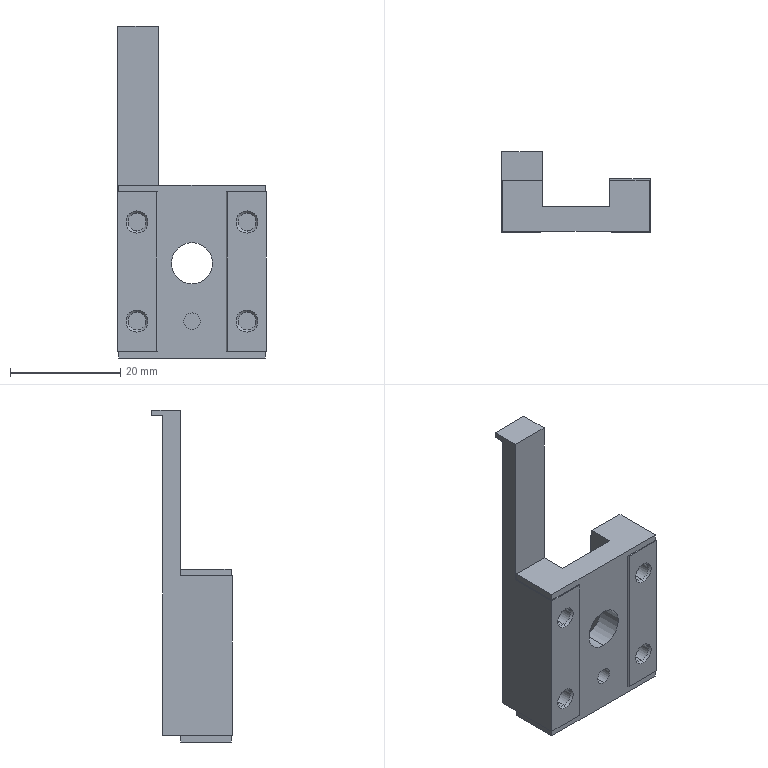Part | STEP file | MHF2-16D1_32-02-CC | 1 solid | 54 faces | box 27 x 14.6 x 60.3 mm | volume 7195 mm3 | plane 34 | cylinder 12 | cone 8 | commonest cylinder face diameters 3.242 x8 3 x2 7.5 x2